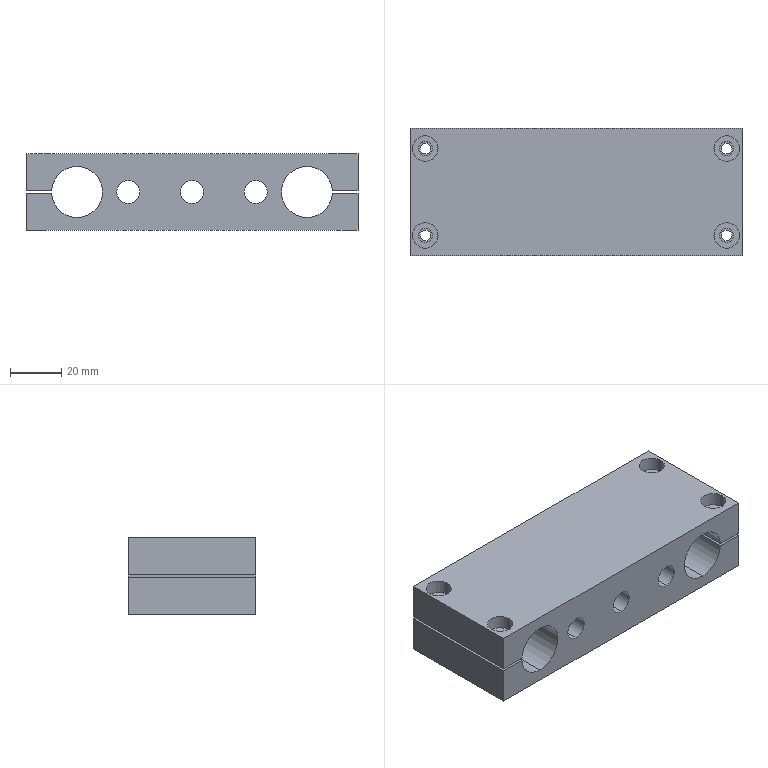Part | STEP file | A13 | 1 solid | 61 faces | box 130 x 50 x 30 mm | volume 142890 mm3 | cylinder 42 | plane 19 | commonest cylinder face diameters 4.2 x8 5.5 x8 10 x8 9 x6 15 x6 20 x6